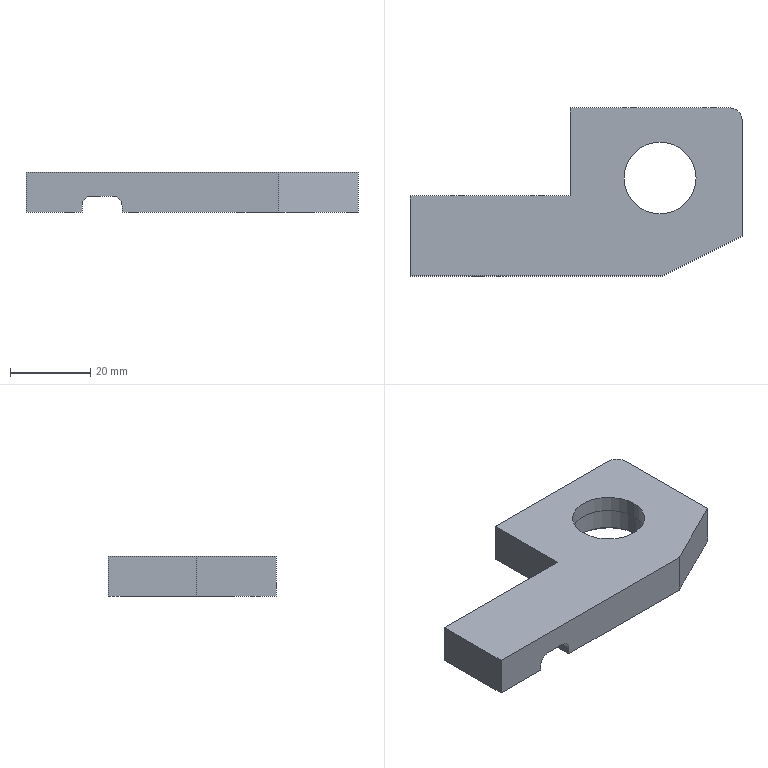Part | NX | features BREP 1 | 1 solid | 47 faces | box 83 x 42 x 10 mm | volume 21101 mm3 | cylinder 19 | cone 14 | plane 14 | commonest cylinder face diameters 3.3 x8 2.5 x4 5 x2 18 x2 19 x2 6 x1
STEP:
#1=CARTESIAN_POINT('',(32.,4.5,-4.5));
#2=VERTEX_POINT('',#1);
#3=CARTESIAN_POINT('',(32.5,4.5,-5.));
#4=VERTEX_POINT('',#3);
#5=CARTESIAN_POINT('',(32.5,4.5,-5.));
#6=DIRECTION('',(0.7071,0.,-0.7071));
#7=VECTOR('',#6,1000.);
#8=LINE('',#5,#7);
#9=EDGE_CURVE('',#2,#4,#8,.T.);
#10=ORIENTED_EDGE('',*,*,#9,.F.);
#11=CARTESIAN_POINT('',(13.,4.5,-4.5));
#12=VERTEX_POINT('',#11);
#13=CARTESIAN_POINT('',(22.5,4.5,-4.5));
#14=DIRECTION('',(0.,0.,-1.));
#15=DIRECTION('',(1.,0.,0.));
#16=AXIS2_PLACEMENT_3D('',#13,#14,#15);
#17=CIRCLE('',#16,9.5);
#18=EDGE_CURVE('',#12,#2,#17,.T.);
#19=ORIENTED_EDGE('',*,*,#18,.F.);
#20=CARTESIAN_POINT('',(12.5,4.5,-5.));
#21=VERTEX_POINT('',#20);
#22=CARTESIAN_POINT('',(12.5,4.5,-5.));
#23=DIRECTION('',(-0.7071,0.,-0.7071));
#24=VECTOR('',#23,1000.);
#25=LINE('',#22,#24);
#26=EDGE_CURVE('',#12,#21,#25,.T.);
#27=ORIENTED_EDGE('',*,*,#26,.T.);
#28=CARTESIAN_POINT('',(22.5,4.5,-5.));
#29=DIRECTION('',(0.,0.,1.));
#30=DIRECTION('',(1.,0.,0.));
#31=AXIS2_PLACEMENT_3D('',#28,#29,#30);
#32=CIRCLE('',#31,10.);
#33=EDGE_CURVE('',#4,#21,#32,.T.);
#34=ORIENTED_EDGE('',*,*,#33,.F.);
#35=EDGE_LOOP('',(#10,#19,#27,#34));
#36=FACE_BOUND('',#35,.T.);
#37=CARTESIAN_POINT('',(22.5,4.5,-5.));
#38=DIRECTION('',(0.,0.,-1.));
#39=DIRECTION('',(-1.,0.,0.));
#40=AXIS2_PLACEMENT_3D('',#37,#38,#39);
#41=CONICAL_SURFACE('',#40,10.,0.7854);
#42=ADVANCED_FACE('',(#36),#41,.F.);
#43=CARTESIAN_POINT('',(-11.75,-15.,2.5));
#44=VERTEX_POINT('',#43);
#45=CARTESIAN_POINT('',(-11.75,-15.,-5.));
#46=VERTEX_POINT('',#45);
#47=CARTESIAN_POINT('',(-11.75,-15.,-5.));
#48=DIRECTION('',(0.,0.,-1.));
#49=VECTOR('',#48,1000.);
#50=LINE('',#47,#49);
#51=EDGE_CURVE('',#44,#46,#50,.T.);
#52=ORIENTED_EDGE('',*,*,#51,.F.);
#53=CARTESIAN_POINT('',(-14.25,-15.,2.5));
#54=VERTEX_POINT('',#53);
#55=CARTESIAN_POINT('',(-13.,-15.,2.5));
#56=DIRECTION('',(0.,0.,-1.));
#57=DIRECTION('',(-1.,0.,0.));
#58=AXIS2_PLACEMENT_3D('',#55,#56,#57);
#59=CIRCLE('',#58,1.25);
#60=EDGE_CURVE('',#54,#44,#59,.T.);
#61=ORIENTED_EDGE('',*,*,#60,.F.);
#62=CARTESIAN_POINT('',(-14.25,-15.,-5.));
#63=VERTEX_POINT('',#62);
#64=CARTESIAN_POINT('',(-14.25,-15.,-5.));
#65=DIRECTION('',(0.,0.,-1.));
#66=VECTOR('',#65,1000.);
#67=LINE('',#64,#66);
#68=EDGE_CURVE('',#54,#63,#67,.T.);
#69=ORIENTED_EDGE('',*,*,#68,.T.);
#70=CARTESIAN_POINT('',(-13.,-15.,-5.));
#71=DIRECTION('',(0.,0.,-1.));
#72=DIRECTION('',(-1.,0.,0.));
#73=AXIS2_PLACEMENT_3D('',#70,#71,#72);
#74=CIRCLE('',#73,1.25);
#75=EDGE_CURVE('',#63,#46,#74,.T.);
#76=ORIENTED_EDGE('',*,*,#75,.T.);
#77=EDGE_LOOP('',(#52,#61,#69,#76));
#78=FACE_BOUND('',#77,.T.);
#79=CARTESIAN_POINT('',(-13.,-15.,-5.));
#80=DIRECTION('',(0.,0.,-1.));
#81=DIRECTION('',(-1.,0.,0.));
#82=AXIS2_PLACEMENT_3D('',#79,#80,#81);
#83=CYLINDRICAL_SURFACE('',#82,1.25);
#84=ADVANCED_FACE('',(#78),#83,.F.);
#85=CARTESIAN_POINT('',(-13.,-15.,3.251));
#86=VERTEX_POINT('',#85);
#87=CARTESIAN_POINT('',(-11.75,-15.,2.5));
#88=DIRECTION('',(0.8572,0.,-0.515));
#89=VECTOR('',#88,1000.);
#90=LINE('',#87,#89);
#91=EDGE_CURVE('',#44,#86,#90,.F.);
#92=ORIENTED_EDGE('',*,*,#91,.T.);
#93=CARTESIAN_POINT('',(-14.25,-15.,2.5));
#94=DIRECTION('',(-0.8572,0.,-0.515));
#95=VECTOR('',#94,1000.);
#96=LINE('',#93,#95);
#97=EDGE_CURVE('',#54,#86,#96,.F.);
#98=ORIENTED_EDGE('',*,*,#97,.F.);
#99=ORIENTED_EDGE('',*,*,#60,.T.);
#100=EDGE_LOOP('',(#92,#98,#99));
#101=FACE_BOUND('',#100,.T.);
#102=CARTESIAN_POINT('',(-13.,-15.,2.5));
#103=DIRECTION('',(0.,0.,-1.));
#104=DIRECTION('',(-1.,0.,0.));
#105=AXIS2_PLACEMENT_3D('',#102,#103,#104);
#106=CONICAL_SURFACE('',#105,1.25,1.03);
#107=ADVANCED_FACE('',(#101),#106,.F.);
#108=CARTESIAN_POINT('',(-27.75,-15.,2.5));
#109=VERTEX_POINT('',#108);
#110=CARTESIAN_POINT('',(-27.75,-15.,-5.));
#111=VERTEX_POINT('',#110);
#112=CARTESIAN_POINT('',(-27.75,-15.,-5.));
#113=DIRECTION('',(0.,0.,-1.));
#114=VECTOR('',#113,1000.);
#115=LINE('',#112,#114);
#116=EDGE_CURVE('',#109,#111,#115,.T.);
#117=ORIENTED_EDGE('',*,*,#116,.F.);
#118=CARTESIAN_POINT('',(-30.25,-15.,2.5));
#119=VERTEX_POINT('',#118);
#120=CARTESIAN_POINT('',(-29.,-15.,2.5));
#121=DIRECTION('',(0.,0.,-1.));
#122=DIRECTION('',(-1.,0.,0.));
#123=AXIS2_PLACEMENT_3D('',#120,#121,#122);
#124=CIRCLE('',#123,1.25);
#125=EDGE_CURVE('',#119,#109,#124,.T.);
#126=ORIENTED_EDGE('',*,*,#125,.F.);
#127=CARTESIAN_POINT('',(-30.25,-15.,-5.));
#128=VERTEX_POINT('',#127);
#129=CARTESIAN_POINT('',(-30.25,-15.,-5.));
#130=DIRECTION('',(0.,0.,-1.));
#131=VECTOR('',#130,1000.);
#132=LINE('',#129,#131);
#133=EDGE_CURVE('',#119,#128,#132,.T.);
#134=ORIENTED_EDGE('',*,*,#133,.T.);
#135=CARTESIAN_POINT('',(-29.,-15.,-5.));
#136=DIRECTION('',(0.,0.,-1.));
#137=DIRECTION('',(-1.,0.,0.));
#138=AXIS2_PLACEMENT_3D('',#135,#136,#137);
#139=CIRCLE('',#138,1.25);
#140=EDGE_CURVE('',#128,#111,#139,.T.);
#141=ORIENTED_EDGE('',*,*,#140,.T.);
#142=EDGE_LOOP('',(#117,#126,#134,#141));
#143=FACE_BOUND('',#142,.T.);
#144=CARTESIAN_POINT('',(-29.,-15.,-5.));
#145=DIRECTION('',(0.,0.,-1.));
#146=DIRECTION('',(-1.,0.,0.));
#147=AXIS2_PLACEMENT_3D('',#144,#145,#146);
#148=CYLINDRICAL_SURFACE('',#147,1.25);
#149=ADVANCED_FACE('',(#143),#148,.F.);
#150=CARTESIAN_POINT('',(-29.,-15.,3.251));
#151=VERTEX_POINT('',#150);
#152=CARTESIAN_POINT('',(-27.75,-15.,2.5));
#153=DIRECTION('',(0.8572,0.,-0.515));
#154=VECTOR('',#153,1000.);
#155=LINE('',#152,#154);
#156=EDGE_CURVE('',#109,#151,#155,.F.);
#157=ORIENTED_EDGE('',*,*,#156,.T.);
#158=CARTESIAN_POINT('',(-30.25,-15.,2.5));
#159=DIRECTION('',(-0.8572,0.,-0.515));
#160=VECTOR('',#159,1000.);
#161=LINE('',#158,#160);
#162=EDGE_CURVE('',#119,#151,#161,.F.);
#163=ORIENTED_EDGE('',*,*,#162,.F.);
#164=ORIENTED_EDGE('',*,*,#125,.T.);
#165=EDGE_LOOP('',(#157,#163,#164));
#166=FACE_BOUND('',#165,.T.);
#167=CARTESIAN_POINT('',(-29.,-15.,2.5));
#168=DIRECTION('',(0.,0.,-1.));
#169=DIRECTION('',(-1.,0.,0.));
#170=AXIS2_PLACEMENT_3D('',#167,#168,#169);
#171=CONICAL_SURFACE('',#170,1.25,1.03);
#172=ADVANCED_FACE('',(#166),#171,.F.);
#173=CARTESIAN_POINT('',(-26.,0.,-3.5));
#174=VERTEX_POINT('',#173);
#175=CARTESIAN_POINT('',(-23.5,0.,-1.));
#176=VERTEX_POINT('',#175);
#177=CARTESIAN_POINT('',(-23.5,0.,-3.5));
#178=DIRECTION('',(0.,1.,0.));
#179=DIRECTION('',(0.,0.,-1.));
#180=AXIS2_PLACEMENT_3D('',#177,#178,#179);
#181=CIRCLE('',#180,2.5);
#182=EDGE_CURVE('',#174,#176,#181,.T.);
#183=ORIENTED_EDGE('',*,*,#182,.T.);
#184=CARTESIAN_POINT('',(-23.5,-20.,-1.));
#185=VERTEX_POINT('',#184);
#186=CARTESIAN_POINT('',(-23.5,-20.,-1.));
#187=DIRECTION('',(0.,1.,0.));
#188=VECTOR('',#187,1000.);
#189=LINE('',#186,#188);
#190=EDGE_CURVE('',#185,#176,#189,.T.);
#191=ORIENTED_EDGE('',*,*,#190,.F.);
#192=CARTESIAN_POINT('',(-26.,-20.,-3.5));
#193=VERTEX_POINT('',#192);
#194=CARTESIAN_POINT('',(-23.5,-20.,-3.5));
#195=DIRECTION('',(0.,1.,0.));
#196=DIRECTION('',(0.,0.,-1.));
#197=AXIS2_PLACEMENT_3D('',#194,#195,#196);
#198=CIRCLE('',#197,2.5);
#199=EDGE_CURVE('',#193,#185,#198,.T.);
#200=ORIENTED_EDGE('',*,*,#199,.F.);
#201=CARTESIAN_POINT('',(-26.,-20.,-3.5));
#202=DIRECTION('',(0.,1.,0.));
#203=VECTOR('',#202,1000.);
#204=LINE('',#201,#203);
#205=EDGE_CURVE('',#193,#174,#204,.T.);
#206=ORIENTED_EDGE('',*,*,#205,.T.);
#207=EDGE_LOOP('',(#183,#191,#200,#206));
#208=FACE_BOUND('',#207,.T.);
#209=CARTESIAN_POINT('',(-23.5,-20.,-3.5));
#210=DIRECTION('',(0.,1.,0.));
#211=DIRECTION('',(0.,0.,1.));
#212=AXIS2_PLACEMENT_3D('',#209,#210,#211);
#213=CYLINDRICAL_SURFACE('',#212,2.5);
#214=ADVANCED_FACE('',(#208),#213,.F.);
#215=CARTESIAN_POINT('',(-18.5,0.,-1.));
#216=VERTEX_POINT('',#215);
#217=CARTESIAN_POINT('',(-18.5,0.,-1.));
#218=DIRECTION('',(1.,0.,0.));
#219=VECTOR('',#218,1000.);
#220=LINE('',#217,#219);
#221=EDGE_CURVE('',#176,#216,#220,.T.);
#222=ORIENTED_EDGE('',*,*,#221,.T.);
#223=CARTESIAN_POINT('',(-18.5,-20.,-1.));
#224=VERTEX_POINT('',#223);
#225=CARTESIAN_POINT('',(-18.5,-20.,-1.));
#226=DIRECTION('',(0.,1.,0.));
#227=VECTOR('',#226,1000.);
#228=LINE('',#225,#227);
#229=EDGE_CURVE('',#224,#216,#228,.T.);
#230=ORIENTED_EDGE('',*,*,#229,.F.);
#231=CARTESIAN_POINT('',(-18.5,-20.,-1.));
#232=DIRECTION('',(1.,0.,0.));
#233=VECTOR('',#232,1000.);
#234=LINE('',#231,#233);
#235=EDGE_CURVE('',#185,#224,#234,.T.);
#236=ORIENTED_EDGE('',*,*,#235,.F.);
#237=ORIENTED_EDGE('',*,*,#190,.T.);
#238=EDGE_LOOP('',(#222,#230,#236,#237));
#239=FACE_BOUND('',#238,.T.);
#240=CARTESIAN_POINT('',(-18.5,-20.,-1.));
#241=DIRECTION('',(0.,0.,1.));
#242=DIRECTION('',(1.,0.,0.));
#243=AXIS2_PLACEMENT_3D('',#240,#241,#242);
#244=PLANE('',#243);
#245=ADVANCED_FACE('',(#239),#244,.F.);
#246=CARTESIAN_POINT('',(-16.,0.,-3.5));
#247=VERTEX_POINT('',#246);
#248=CARTESIAN_POINT('',(-18.5,0.,-3.5));
#249=DIRECTION('',(0.,1.,0.));
#250=DIRECTION('',(0.,0.,-1.));
#251=AXIS2_PLACEMENT_3D('',#248,#249,#250);
#252=CIRCLE('',#251,2.5);
#253=EDGE_CURVE('',#216,#247,#252,.T.);
#254=ORIENTED_EDGE('',*,*,#253,.T.);
#255=CARTESIAN_POINT('',(-16.,-20.,-3.5));
#256=VERTEX_POINT('',#255);
#257=CARTESIAN_POINT('',(-16.,-20.,-3.5));
#258=DIRECTION('',(0.,1.,0.));
#259=VECTOR('',#258,1000.);
#260=LINE('',#257,#259);
#261=EDGE_CURVE('',#256,#247,#260,.T.);
#262=ORIENTED_EDGE('',*,*,#261,.F.);
#263=CARTESIAN_POINT('',(-18.5,-20.,-3.5));
#264=DIRECTION('',(0.,1.,0.));
#265=DIRECTION('',(0.,0.,-1.));
#266=AXIS2_PLACEMENT_3D('',#263,#264,#265);
#267=CIRCLE('',#266,2.5);
#268=EDGE_CURVE('',#224,#256,#267,.T.);
#269=ORIENTED_EDGE('',*,*,#268,.F.);
#270=ORIENTED_EDGE('',*,*,#229,.T.);
#271=EDGE_LOOP('',(#254,#262,#269,#270));
#272=FACE_BOUND('',#271,.T.);
#273=CARTESIAN_POINT('',(-18.5,-20.,-3.5));
#274=DIRECTION('',(0.,1.,0.));
#275=DIRECTION('',(0.,0.,1.));
#276=AXIS2_PLACEMENT_3D('',#273,#274,#275);
#277=CYLINDRICAL_SURFACE('',#276,2.5);
#278=ADVANCED_FACE('',(#272),#277,.F.);
#279=CARTESIAN_POINT('',(-26.,0.,-5.));
#280=VERTEX_POINT('',#279);
#281=CARTESIAN_POINT('',(-26.,0.,-9.));
#282=DIRECTION('',(0.,0.,1.));
#283=VECTOR('',#282,1000.);
#284=LINE('',#281,#283);
#285=EDGE_CURVE('',#280,#174,#284,.T.);
#286=ORIENTED_EDGE('',*,*,#285,.T.);
#287=ORIENTED_EDGE('',*,*,#205,.F.);
#288=CARTESIAN_POINT('',(-26.,-20.,-5.));
#289=VERTEX_POINT('',#288);
#290=CARTESIAN_POINT('',(-26.,-20.,-9.));
#291=DIRECTION('',(0.,0.,1.));
#292=VECTOR('',#291,1000.);
#293=LINE('',#290,#292);
#294=EDGE_CURVE('',#289,#193,#293,.T.);
#295=ORIENTED_EDGE('',*,*,#294,.F.);
#296=CARTESIAN_POINT('',(-26.,0.,-5.));
#297=DIRECTION('',(0.,-1.,0.));
#298=VECTOR('',#297,1000.);
#299=LINE('',#296,#298);
#300=EDGE_CURVE('',#280,#289,#299,.T.);
#301=ORIENTED_EDGE('',*,*,#300,.F.);
#302=EDGE_LOOP('',(#286,#287,#295,#301));
#303=FACE_BOUND('',#302,.T.);
#304=CARTESIAN_POINT('',(-26.,-20.,-9.));
#305=DIRECTION('',(-1.,0.,0.));
#306=DIRECTION('',(0.,0.,1.));
#307=AXIS2_PLACEMENT_3D('',#304,#305,#306);
#308=PLANE('',#307);
#309=ADVANCED_FACE('',(#303),#308,.F.);
#310=CARTESIAN_POINT('',(-16.,-20.,-5.));
#311=VERTEX_POINT('',#310);
#312=CARTESIAN_POINT('',(-16.,-20.,-9.));
#313=DIRECTION('',(0.,0.,-1.));
#314=VECTOR('',#313,1000.);
#315=LINE('',#312,#314);
#316=EDGE_CURVE('',#256,#311,#315,.T.);
#317=ORIENTED_EDGE('',*,*,#316,.F.);
#318=ORIENTED_EDGE('',*,*,#261,.T.);
#319=CARTESIAN_POINT('',(-16.,0.,-5.));
#320=VERTEX_POINT('',#319);
#321=CARTESIAN_POINT('',(-16.,0.,-9.));
#322=DIRECTION('',(0.,0.,-1.));
#323=VECTOR('',#322,1000.);
#324=LINE('',#321,#323);
#325=EDGE_CURVE('',#247,#320,#324,.T.);
#326=ORIENTED_EDGE('',*,*,#325,.T.);
#327=CARTESIAN_POINT('',(-16.,0.,-5.));
#328=DIRECTION('',(0.,1.,0.));
#329=VECTOR('',#328,1000.);
#330=LINE('',#327,#329);
#331=EDGE_CURVE('',#311,#320,#330,.T.);
#332=ORIENTED_EDGE('',*,*,#331,.F.);
#333=EDGE_LOOP('',(#317,#318,#326,#332));
#334=FACE_BOUND('',#333,.T.);
#335=CARTESIAN_POINT('',(-16.,-20.,-9.));
#336=DIRECTION('',(1.,0.,0.));
#337=DIRECTION('',(0.,0.,-1.));
#338=AXIS2_PLACEMENT_3D('',#335,#336,#337);
#339=PLANE('',#338);
#340=ADVANCED_FACE('',(#334),#339,.F.);
#341=CARTESIAN_POINT('',(35.,22.,-1.65));
#342=VERTEX_POINT('',#341);
#343=CARTESIAN_POINT('',(35.,11.9,-1.65));
#344=VERTEX_POINT('',#343);
#345=CARTESIAN_POINT('',(35.,22.,-1.65));
#346=DIRECTION('',(0.,1.,0.));
#347=VECTOR('',#346,1000.);
#348=LINE('',#345,#347);
#349=EDGE_CURVE('',#342,#344,#348,.F.);
#350=ORIENTED_EDGE('',*,*,#349,.T.);
#351=CARTESIAN_POINT('',(35.,11.9,1.65));
#352=VERTEX_POINT('',#351);
#353=CARTESIAN_POINT('',(35.,11.9,0.));
#354=DIRECTION('',(0.,1.,0.));
#355=DIRECTION('',(0.,0.,1.));
#356=AXIS2_PLACEMENT_3D('',#353,#354,#355);
#357=CIRCLE('',#356,1.65);
#358=EDGE_CURVE('',#352,#344,#357,.T.);
#359=ORIENTED_EDGE('',*,*,#358,.F.);
#360=CARTESIAN_POINT('',(35.,22.,1.65));
#361=VERTEX_POINT('',#360);
#362=CARTESIAN_POINT('',(35.,22.,1.65));
#363=DIRECTION('',(0.,1.,0.));
#364=VECTOR('',#363,1000.);
#365=LINE('',#362,#364);
#366=EDGE_CURVE('',#361,#352,#365,.F.);
#367=ORIENTED_EDGE('',*,*,#366,.F.);
#368=CARTESIAN_POINT('',(35.,22.,0.));
#369=DIRECTION('',(0.,1.,0.));
#370=DIRECTION('',(0.,0.,1.));
#371=AXIS2_PLACEMENT_3D('',#368,#369,#370);
#372=CIRCLE('',#371,1.65);
#373=EDGE_CURVE('',#361,#342,#372,.T.);
#374=ORIENTED_EDGE('',*,*,#373,.T.);
#375=EDGE_LOOP('',(#350,#359,#367,#374));
#376=FACE_BOUND('',#375,.T.);
#377=CARTESIAN_POINT('',(35.,22.,0.));
#378=DIRECTION('',(0.,1.,0.));
#379=DIRECTION('',(0.,0.,1.));
#380=AXIS2_PLACEMENT_3D('',#377,#378,#379);
#381=CYLINDRICAL_SURFACE('',#380,1.65);
#382=ADVANCED_FACE('',(#376),#381,.F.);
#383=CARTESIAN_POINT('',(35.,10.909,0.));
#384=VERTEX_POINT('',#383);
#385=CARTESIAN_POINT('',(35.,11.9,-1.65));
#386=DIRECTION('',(0.,0.515,-0.8572));
#387=VECTOR('',#386,1000.);
#388=LINE('',#385,#387);
#389=EDGE_CURVE('',#384,#344,#388,.T.);
#390=ORIENTED_EDGE('',*,*,#389,.F.);
#391=CARTESIAN_POINT('',(35.,11.9,1.65));
#392=DIRECTION('',(0.,0.515,0.8572));
#393=VECTOR('',#392,1000.);
#394=LINE('',#391,#393);
#395=EDGE_CURVE('',#384,#352,#394,.T.);
#396=ORIENTED_EDGE('',*,*,#395,.T.);
#397=ORIENTED_EDGE('',*,*,#358,.T.);
#398=EDGE_LOOP('',(#390,#396,#397));
#399=FACE_BOUND('',#398,.T.);
#400=CARTESIAN_POINT('',(35.,11.9,0.));
#401=DIRECTION('',(0.,1.,0.));
#402=DIRECTION('',(0.,0.,1.));
#403=AXIS2_PLACEMENT_3D('',#400,#401,#402);
#404=CONICAL_SURFACE('',#403,1.65,1.03);
#405=ADVANCED_FACE('',(#399),#404,.F.);
#406=CARTESIAN_POINT('',(15.,22.,-1.65));
#407=VERTEX_POINT('',#406);
#408=CARTESIAN_POINT('',(15.,11.9,-1.65));
#409=VERTEX_POINT('',#408);
#410=CARTESIAN_POINT('',(15.,22.,-1.65));
#411=DIRECTION('',(0.,1.,0.));
#412=VECTOR('',#411,1000.);
#413=LINE('',#410,#412);
#414=EDGE_CURVE('',#407,#409,#413,.F.);
#415=ORIENTED_EDGE('',*,*,#414,.T.);
#416=CARTESIAN_POINT('',(16.543,11.9,-0.5854));
#417=VERTEX_POINT('',#416);
#418=CARTESIAN_POINT('',(15.,11.9,0.));
#419=DIRECTION('',(0.,1.,0.));
#420=DIRECTION('',(0.,0.,1.));
#421=AXIS2_PLACEMENT_3D('',#418,#419,#420);
#422=CIRCLE('',#421,1.65);
#423=EDGE_CURVE('',#417,#409,#422,.T.);
#424=ORIENTED_EDGE('',*,*,#423,.F.);
#425=CARTESIAN_POINT('',(16.543,11.9,0.5854));
#426=VERTEX_POINT('',#425);
#427=CARTESIAN_POINT('',(16.543,11.9,-0.5854));
#428=CARTESIAN_POINT('',(16.684,12.014,-0.2124));
#429=CARTESIAN_POINT('',(16.684,12.014,0.2124));
#430=CARTESIAN_POINT('',(16.543,11.9,0.5854));
#431=B_SPLINE_CURVE_WITH_KNOTS('',3,(#427,#428,#429,#430),.UNSPECIFIED.,.F.,.F.,(4,4),(0.,1.),.UNSPECIFIED.);
#432=EDGE_CURVE('',#417,#426,#431,.T.);
#433=ORIENTED_EDGE('',*,*,#432,.T.);
#434=CARTESIAN_POINT('',(15.,11.9,1.65));
#435=VERTEX_POINT('',#434);
#436=CARTESIAN_POINT('',(15.,11.9,0.));
#437=DIRECTION('',(0.,1.,0.));
#438=DIRECTION('',(0.,0.,1.));
#439=AXIS2_PLACEMENT_3D('',#436,#437,#438);
#440=CIRCLE('',#439,1.65);
#441=EDGE_CURVE('',#435,#426,#440,.T.);
#442=ORIENTED_EDGE('',*,*,#441,.F.);
#443=CARTESIAN_POINT('',(15.,22.,1.65));
#444=VERTEX_POINT('',#443);
#445=CARTESIAN_POINT('',(15.,22.,1.65));
#446=DIRECTION('',(0.,1.,0.));
#447=VECTOR('',#446,1000.);
#448=LINE('',#445,#447);
#449=EDGE_CURVE('',#444,#435,#448,.F.);
#450=ORIENTED_EDGE('',*,*,#449,.F.);
#451=CARTESIAN_POINT('',(15.,22.,0.));
#452=DIRECTION('',(0.,1.,0.));
#453=DIRECTION('',(0.,0.,1.));
#454=AXIS2_PLACEMENT_3D('',#451,#452,#453);
#455=CIRCLE('',#454,1.65);
#456=EDGE_CURVE('',#444,#407,#455,.T.);
#457=ORIENTED_EDGE('',*,*,#456,.T.);
#458=EDGE_LOOP('',(#415,#424,#433,#442,#450,#457));
#459=FACE_BOUND('',#458,.T.);
#460=CARTESIAN_POINT('',(15.,22.,0.));
#461=DIRECTION('',(0.,1.,0.));
#462=DIRECTION('',(0.,0.,1.));
#463=AXIS2_PLACEMENT_3D('',#460,#461,#462);
#464=CYLINDRICAL_SURFACE('',#463,1.65);
#465=ADVANCED_FACE('',(#459),#464,.F.);
#466=CARTESIAN_POINT('',(15.,10.909,0.));
#467=VERTEX_POINT('',#466);
#468=CARTESIAN_POINT('',(15.,11.9,-1.65));
#469=DIRECTION('',(0.,0.515,-0.8572));
#470=VECTOR('',#469,1000.);
#471=LINE('',#468,#470);
#472=EDGE_CURVE('',#467,#409,#471,.T.);
#473=ORIENTED_EDGE('',*,*,#472,.F.);
#474=CARTESIAN_POINT('',(15.,11.9,1.65));
#475=DIRECTION('',(0.,0.515,0.8572));
#476=VECTOR('',#475,1000.);
#477=LINE('',#474,#476);
#478=EDGE_CURVE('',#467,#435,#477,.T.);
#479=ORIENTED_EDGE('',*,*,#478,.T.);
#480=ORIENTED_EDGE('',*,*,#441,.T.);
#481=CARTESIAN_POINT('',(16.543,11.9,-0.5854));
#482=CARTESIAN_POINT('',(16.39,11.777,-0.4109));
#483=CARTESIAN_POINT('',(16.149,11.566,-0.001288));
#484=CARTESIAN_POINT('',(16.389,11.776,0.4098));
#485=CARTESIAN_POINT('',(16.543,11.9,0.5854));
#486=B_SPLINE_CURVE_WITH_KNOTS('',3,(#481,#482,#483,#484,#485),.UNSPECIFIED.,.F.,.F.,(4,1,4),(0.,0.5,1.),.UNSPECIFIED.);
#487=EDGE_CURVE('',#426,#417,#486,.F.);
#488=ORIENTED_EDGE('',*,*,#487,.T.);
#489=ORIENTED_EDGE('',*,*,#423,.T.);
#490=EDGE_LOOP('',(#473,#479,#480,#488,#489));
#491=FACE_BOUND('',#490,.T.);
#492=CARTESIAN_POINT('',(15.,11.9,0.));
#493=DIRECTION('',(0.,1.,0.));
#494=DIRECTION('',(0.,0.,1.));
#495=AXIS2_PLACEMENT_3D('',#492,#493,#494);
#496=CONICAL_SURFACE('',#495,1.65,1.03);
#497=ADVANCED_FACE('',(#491),#496,.F.);
#498=CARTESIAN_POINT('',(43.,19.,5.));
#499=VERTEX_POINT('',#498);
#500=CARTESIAN_POINT('',(40.,22.,5.));
#501=VERTEX_POINT('',#500);
#502=CARTESIAN_POINT('',(40.,19.,5.));
#503=DIRECTION('',(0.,0.,1.));
#504=DIRECTION('',(1.,0.,0.));
#505=AXIS2_PLACEMENT_3D('',#502,#503,#504);
#506=CIRCLE('',#505,3.);
#507=EDGE_CURVE('',#499,#501,#506,.T.);
#508=ORIENTED_EDGE('',*,*,#507,.F.);
#509=CARTESIAN_POINT('',(43.,19.,-5.));
#510=VERTEX_POINT('',#509);
#511=CARTESIAN_POINT('',(43.,19.,5.));
#512=DIRECTION('',(0.,0.,1.));
#513=VECTOR('',#512,1000.);
#514=LINE('',#511,#513);
#515=EDGE_CURVE('',#510,#499,#514,.T.);
#516=ORIENTED_EDGE('',*,*,#515,.F.);
#517=CARTESIAN_POINT('',(40.,22.,-5.));
#518=VERTEX_POINT('',#517);
#519=CARTESIAN_POINT('',(40.,19.,-5.));
#520=DIRECTION('',(0.,0.,-1.));
#521=DIRECTION('',(1.,0.,0.));
#522=AXIS2_PLACEMENT_3D('',#519,#520,#521);
#523=CIRCLE('',#522,3.);
#524=EDGE_CURVE('',#518,#510,#523,.T.);
#525=ORIENTED_EDGE('',*,*,#524,.F.);
#526=CARTESIAN_POINT('',(40.,22.,5.));
#527=DIRECTION('',(0.,0.,-1.));
#528=VECTOR('',#527,1000.);
#529=LINE('',#526,#528);
#530=EDGE_CURVE('',#501,#518,#529,.T.);
#531=ORIENTED_EDGE('',*,*,#530,.F.);
#532=EDGE_LOOP('',(#508,#516,#525,#531));
#533=FACE_BOUND('',#532,.T.);
#534=CARTESIAN_POINT('',(40.,19.,5.));
#535=DIRECTION('',(0.,0.,-1.));
#536=DIRECTION('',(-1.,0.,0.));
#537=AXIS2_PLACEMENT_3D('',#534,#535,#536);
#538=CYLINDRICAL_SURFACE('',#537,3.);
#539=ADVANCED_FACE('',(#533),#538,.T.);
#540=CARTESIAN_POINT('',(13.5,4.5,5.));
#541=VERTEX_POINT('',#540);
#542=CARTESIAN_POINT('',(13.5,4.5,1.));
#543=VERTEX_POINT('',#542);
#544=CARTESIAN_POINT('',(13.5,4.5,-5.));
#545=DIRECTION('',(0.,0.,1.));
#546=VECTOR('',#545,1000.);
#547=LINE('',#544,#546);
#548=EDGE_CURVE('',#541,#543,#547,.F.);
#549=ORIENTED_EDGE('',*,*,#548,.T.);
#550=CARTESIAN_POINT('',(31.5,4.5,1.));
#551=VERTEX_POINT('',#550);
#552=CARTESIAN_POINT('',(22.5,4.5,1.));
#553=DIRECTION('',(0.,0.,1.));
#554=DIRECTION('',(1.,0.,0.));
#555=AXIS2_PLACEMENT_3D('',#552,#553,#554);
#556=CIRCLE('',#555,9.);
#557=EDGE_CURVE('',#551,#543,#556,.T.);
#558=ORIENTED_EDGE('',*,*,#557,.F.);
#559=CARTESIAN_POINT('',(31.5,4.5,5.));
#560=VERTEX_POINT('',#559);
#561=CARTESIAN_POINT('',(31.5,4.5,-5.));
#562=DIRECTION('',(0.,0.,1.));
#563=VECTOR('',#562,1000.);
#564=LINE('',#561,#563);
#565=EDGE_CURVE('',#560,#551,#564,.F.);
#566=ORIENTED_EDGE('',*,*,#565,.F.);
#567=CARTESIAN_POINT('',(22.5,4.5,5.));
#568=DIRECTION('',(0.,0.,1.));
#569=DIRECTION('',(1.,0.,0.));
#570=AXIS2_PLACEMENT_3D('',#567,#568,#569);
#571=CIRCLE('',#570,9.);
#572=EDGE_CURVE('',#560,#541,#571,.T.);
#573=ORIENTED_EDGE('',*,*,#572,.T.);
#574=EDGE_LOOP('',(#549,#558,#566,#573));
#575=FACE_BOUND('',#574,.T.);
#576=CARTESIAN_POINT('',(22.5,4.5,-5.));
#577=DIRECTION('',(0.,0.,1.));
#578=DIRECTION('',(1.,0.,0.));
#579=AXIS2_PLACEMENT_3D('',#576,#577,#578);
#580=CYLINDRICAL_SURFACE('',#579,9.);
#581=ADVANCED_FACE('',(#575),#580,.F.);
#582=CARTESIAN_POINT('',(13.,4.5,1.));
#583=VERTEX_POINT('',#582);
#584=CARTESIAN_POINT('',(32.,4.5,1.));
#585=VERTEX_POINT('',#584);
#586=CARTESIAN_POINT('',(22.5,4.5,1.));
#587=DIRECTION('',(0.,0.,1.));
#588=DIRECTION('',(1.,0.,0.));
#589=AXIS2_PLACEMENT_3D('',#586,#587,#588);
#590=CIRCLE('',#589,9.5);
#591=EDGE_CURVE('',#583,#585,#590,.T.);
#592=ORIENTED_EDGE('',*,*,#591,.F.);
#593=CARTESIAN_POINT('',(22.5,4.5,1.));
#594=DIRECTION('',(0.,0.,1.));
#595=DIRECTION('',(1.,0.,0.));
#596=AXIS2_PLACEMENT_3D('',#593,#594,#595);
#597=CIRCLE('',#596,9.5);
#598=EDGE_CURVE('',#585,#583,#597,.T.);
#599=ORIENTED_EDGE('',*,*,#598,.F.);
#600=EDGE_LOOP('',(#592,#599));
#601=FACE_BOUND('',#600,.T.);
#602=ORIENTED_EDGE('',*,*,#557,.T.);
#603=CARTESIAN_POINT('',(22.5,4.5,1.));
#604=DIRECTION('',(0.,0.,1.));
#605=DIRECTION('',(1.,0.,0.));
#606=AXIS2_PLACEMENT_3D('',#603,#604,#605);
#607=CIRCLE('',#606,9.);
#608=EDGE_CURVE('',#543,#551,#607,.T.);
#609=ORIENTED_EDGE('',*,*,#608,.T.);
#610=EDGE_LOOP('',(#602,#609));
#611=FACE_BOUND('',#610,.T.);
#612=CARTESIAN_POINT('',(22.5,4.5,1.));
#613=DIRECTION('',(0.,0.,1.));
#614=DIRECTION('',(1.,0.,0.));
#615=AXIS2_PLACEMENT_3D('',#612,#613,#614);
#616=PLANE('',#615);
#617=ADVANCED_FACE('',(#601,#611),#616,.F.);
#618=ORIENTED_EDGE('',*,*,#432,.F.);
#619=ORIENTED_EDGE('',*,*,#487,.F.);
#620=EDGE_LOOP('',(#618,#619));
#621=FACE_BOUND('',#620,.T.);
#622=CARTESIAN_POINT('',(32.,4.5,1.));
#623=DIRECTION('',(0.,0.,-1.));
#624=VECTOR('',#623,1000.);
#625=LINE('',#622,#624);
#626=EDGE_CURVE('',#585,#2,#625,.T.);
#627=ORIENTED_EDGE('',*,*,#626,.F.);
#628=ORIENTED_EDGE('',*,*,#598,.T.);
#629=CARTESIAN_POINT('',(13.,4.5,1.));
#630=DIRECTION('',(0.,0.,-1.));
#631=VECTOR('',#630,1000.);
#632=LINE('',#629,#631);
#633=EDGE_CURVE('',#583,#12,#632,.T.);
#634=ORIENTED_EDGE('',*,*,#633,.T.);
#635=ORIENTED_EDGE('',*,*,#18,.T.);
#636=EDGE_LOOP('',(#627,#628,#634,#635));
#637=FACE_BOUND('',#636,.T.);
#638=CARTESIAN_POINT('',(22.5,4.5,1.));
#639=DIRECTION('',(0.,0.,-1.));
#640=DIRECTION('',(-1.,0.,0.));
#641=AXIS2_PLACEMENT_3D('',#638,#639,#640);
#642=CYLINDRICAL_SURFACE('',#641,9.5);
#643=ADVANCED_FACE('',(#621,#637),#642,.F.);
#644=CARTESIAN_POINT('',(23.,-20.,5.));
#645=VERTEX_POINT('',#644);
#646=CARTESIAN_POINT('',(43.,-10.,5.));
#647=VERTEX_POINT('',#646);
#648=CARTESIAN_POINT('',(12.6,-25.2,5.));
#649=DIRECTION('',(0.8944,0.4472,0.));
#650=VECTOR('',#649,1000.);
#651=LINE('',#648,#650);
#652=EDGE_CURVE('',#645,#647,#651,.T.);
#653=ORIENTED_EDGE('',*,*,#652,.F.);
#654=CARTESIAN_POINT('',(23.,-20.,-5.));
#655=VERTEX_POINT('',#654);
#656=CARTESIAN_POINT('',(23.,-20.,5.));
#657=DIRECTION('',(0.,0.,1.));
#658=VECTOR('',#657,1000.);
#659=LINE('',#656,#658);
#660=EDGE_CURVE('',#655,#645,#659,.T.);
#661=ORIENTED_EDGE('',*,*,#660,.F.);
#662=CARTESIAN_POINT('',(43.,-10.,-5.));
#663=VERTEX_POINT('',#662);
#664=CARTESIAN_POINT('',(43.,-10.,-5.));
#665=DIRECTION('',(-0.8944,-0.4472,0.));
#666=VECTOR('',#665,1000.);
#667=LINE('',#664,#666);
#668=EDGE_CURVE('',#663,#655,#667,.T.);
#669=ORIENTED_EDGE('',*,*,#668,.F.);
#670=CARTESIAN_POINT('',(43.,-10.,5.));
#671=DIRECTION('',(0.,0.,-1.));
#672=VECTOR('',#671,1000.);
#673=LINE('',#670,#672);
#674=EDGE_CURVE('',#647,#663,#673,.T.);
#675=ORIENTED_EDGE('',*,*,#674,.F.);
#676=EDGE_LOOP('',(#653,#661,#669,#675));
#677=FACE_BOUND('',#676,.T.);
#678=CARTESIAN_POINT('',(43.,-10.,5.));
#679=DIRECTION('',(-0.4472,0.8944,0.));
#680=DIRECTION('',(0.,0.,-1.));
#681=AXIS2_PLACEMENT_3D('',#678,#679,#680);
#682=PLANE('',#681);
#683=ADVANCED_FACE('',(#677),#682,.F.);
#684=CARTESIAN_POINT('',(-8.,0.,-1.65));
#685=VERTEX_POINT('',#684);
#686=CARTESIAN_POINT('',(-8.,-12.1,-1.65));
#687=VERTEX_POINT('',#686);
#688=CARTESIAN_POINT('',(-8.,0.,-1.65));
#689=DIRECTION('',(0.,1.,0.));
#690=VECTOR('',#689,1000.);
#691=LINE('',#688,#690);
#692=EDGE_CURVE('',#685,#687,#691,.F.);
#693=ORIENTED_EDGE('',*,*,#692,.T.);
#694=CARTESIAN_POINT('',(-8.,-12.1,1.65));
#695=VERTEX_POINT('',#694);
#696=CARTESIAN_POINT('',(-8.,-12.1,0.));
#697=DIRECTION('',(0.,1.,0.));
#698=DIRECTION('',(0.,0.,1.));
#699=AXIS2_PLACEMENT_3D('',#696,#697,#698);
#700=CIRCLE('',#699,1.65);
#701=EDGE_CURVE('',#695,#687,#700,.T.);
#702=ORIENTED_EDGE('',*,*,#701,.F.);
#703=CARTESIAN_POINT('',(-8.,0.,1.65));
#704=VERTEX_POINT('',#703);
#705=CARTESIAN_POINT('',(-8.,0.,1.65));
#706=DIRECTION('',(0.,1.,0.));
#707=VECTOR('',#706,1000.);
#708=LINE('',#705,#707);
#709=EDGE_CURVE('',#704,#695,#708,.F.);
#710=ORIENTED_EDGE('',*,*,#709,.F.);
#711=CARTESIAN_POINT('',(-8.,0.,0.));
#712=DIRECTION('',(0.,1.,0.));
#713=DIRECTION('',(0.,0.,1.));
#714=AXIS2_PLACEMENT_3D('',#711,#712,#713);
#715=CIRCLE('',#714,1.65);
#716=EDGE_CURVE('',#704,#685,#715,.T.);
#717=ORIENTED_EDGE('',*,*,#716,.T.);
#718=EDGE_LOOP('',(#693,#702,#710,#717));
#719=FACE_BOUND('',#718,.T.);
#720=CARTESIAN_POINT('',(-8.,0.,0.));
#721=DIRECTION('',(0.,1.,0.));
#722=DIRECTION('',(0.,0.,1.));
#723=AXIS2_PLACEMENT_3D('',#720,#721,#722);
#724=CYLINDRICAL_SURFACE('',#723,1.65);
#725=ADVANCED_FACE('',(#719),#724,.F.);
#726=CARTESIAN_POINT('',(-8.,-13.091,0.));
#727=VERTEX_POINT('',#726);
#728=CARTESIAN_POINT('',(-8.,-12.1,-1.65));
#729=DIRECTION('',(0.,0.515,-0.8572));
#730=VECTOR('',#729,1000.);
#731=LINE('',#728,#730);
#732=EDGE_CURVE('',#727,#687,#731,.T.);
#733=ORIENTED_EDGE('',*,*,#732,.F.);
#734=CARTESIAN_POINT('',(-8.,-12.1,1.65));
#735=DIRECTION('',(0.,0.515,0.8572));
#736=VECTOR('',#735,1000.);
#737=LINE('',#734,#736);
#738=EDGE_CURVE('',#727,#695,#737,.T.);
#739=ORIENTED_EDGE('',*,*,#738,.T.);
#740=ORIENTED_EDGE('',*,*,#701,.T.);
#741=EDGE_LOOP('',(#733,#739,#740));
#742=FACE_BOUND('',#741,.T.);
#743=CARTESIAN_POINT('',(-8.,-12.1,0.));
#744=DIRECTION('',(0.,1.,0.));
#745=DIRECTION('',(0.,0.,1.));
#746=AXIS2_PLACEMENT_3D('',#743,#744,#745);
#747=CONICAL_SURFACE('',#746,1.65,1.03);
#748=ADVANCED_FACE('',(#742),#747,.F.);
#749=CARTESIAN_POINT('',(-28.,0.,-1.65));
#750=VERTEX_POINT('',#749);
#751=CARTESIAN_POINT('',(-28.,-12.1,-1.65));
#752=VERTEX_POINT('',#751);
#753=CARTESIAN_POINT('',(-28.,0.,-1.65));
#754=DIRECTION('',(0.,1.,0.));
#755=VECTOR('',#754,1000.);
#756=LINE('',#753,#755);
#757=EDGE_CURVE('',#750,#752,#756,.F.);
#758=ORIENTED_EDGE('',*,*,#757,.T.);
#759=CARTESIAN_POINT('',(-28.,-12.1,1.65));
#760=VERTEX_POINT('',#759);
#761=CARTESIAN_POINT('',(-28.,-12.1,0.));
#762=DIRECTION('',(0.,1.,0.));
#763=DIRECTION('',(0.,0.,1.));
#764=AXIS2_PLACEMENT_3D('',#761,#762,#763);
#765=CIRCLE('',#764,1.65);
#766=EDGE_CURVE('',#760,#752,#765,.T.);
#767=ORIENTED_EDGE('',*,*,#766,.F.);
#768=CARTESIAN_POINT('',(-28.,0.,1.65));
#769=VERTEX_POINT('',#768);
#770=CARTESIAN_POINT('',(-28.,0.,1.65));
#771=DIRECTION('',(0.,1.,0.));
#772=VECTOR('',#771,1000.);
#773=LINE('',#770,#772);
#774=EDGE_CURVE('',#769,#760,#773,.F.);
#775=ORIENTED_EDGE('',*,*,#774,.F.);
#776=CARTESIAN_POINT('',(-28.,0.,0.));
#777=DIRECTION('',(0.,1.,0.));
#778=DIRECTION('',(0.,0.,1.));
#779=AXIS2_PLACEMENT_3D('',#776,#777,#778);
#780=CIRCLE('',#779,1.65);
#781=EDGE_CURVE('',#769,#750,#780,.T.);
#782=ORIENTED_EDGE('',*,*,#781,.T.);
#783=EDGE_LOOP('',(#758,#767,#775,#782));
#784=FACE_BOUND('',#783,.T.);
#785=CARTESIAN_POINT('',(-28.,0.,0.));
#786=DIRECTION('',(0.,1.,0.));
#787=DIRECTION('',(0.,0.,1.));
#788=AXIS2_PLACEMENT_3D('',#785,#786,#787);
#789=CYLINDRICAL_SURFACE('',#788,1.65);
#790=ADVANCED_FACE('',(#784),#789,.F.);
#791=CARTESIAN_POINT('',(-28.,-13.091,0.));
#792=VERTEX_POINT('',#791);
#793=CARTESIAN_POINT('',(-28.,-12.1,-1.65));
#794=DIRECTION('',(0.,0.515,-0.8572));
#795=VECTOR('',#794,1000.);
#796=LINE('',#793,#795);
#797=EDGE_CURVE('',#792,#752,#796,.T.);
#798=ORIENTED_EDGE('',*,*,#797,.F.);
#799=CARTESIAN_POINT('',(-28.,-12.1,1.65));
#800=DIRECTION('',(0.,0.515,0.8572));
#801=VECTOR('',#800,1000.);
#802=LINE('',#799,#801);
#803=EDGE_CURVE('',#792,#760,#802,.T.);
#804=ORIENTED_EDGE('',*,*,#803,.T.);
#805=ORIENTED_EDGE('',*,*,#766,.T.);
#806=EDGE_LOOP('',(#798,#804,#805));
#807=FACE_BOUND('',#806,.T.);
#808=CARTESIAN_POINT('',(-28.,-12.1,0.));
#809=DIRECTION('',(0.,1.,0.));
#810=DIRECTION('',(0.,0.,1.));
#811=AXIS2_PLACEMENT_3D('',#808,#809,#810);
#812=CONICAL_SURFACE('',#811,1.65,1.03);
#813=ADVANCED_FACE('',(#807),#812,.F.);
#814=CARTESIAN_POINT('',(-40.,0.,-5.));
#815=VERTEX_POINT('',#814);
#816=CARTESIAN_POINT('',(-40.,0.,-5.));
#817=DIRECTION('',(-1.,0.,0.));
#818=VECTOR('',#817,1000.);
#819=LINE('',#816,#818);
#820=EDGE_CURVE('',#280,#815,#819,.T.);
#821=ORIENTED_EDGE('',*,*,#820,.F.);
#822=ORIENTED_EDGE('',*,*,#300,.T.);
#823=CARTESIAN_POINT('',(-40.,-20.,-5.));
#824=VERTEX_POINT('',#823);
#825=CARTESIAN_POINT('',(43.,-20.,-5.));
#826=DIRECTION('',(1.,0.,0.));
#827=VECTOR('',#826,1000.);
#828=LINE('',#825,#827);
#829=EDGE_CURVE('',#824,#289,#828,.T.);
#830=ORIENTED_EDGE('',*,*,#829,.F.);
#831=CARTESIAN_POINT('',(-40.,-20.,-5.));
#832=DIRECTION('',(0.,-1.,0.));
#833=VECTOR('',#832,1000.);
#834=LINE('',#831,#833);
#835=EDGE_CURVE('',#815,#824,#834,.T.);
#836=ORIENTED_EDGE('',*,*,#835,.F.);
#837=EDGE_LOOP('',(#821,#822,#830,#836));
#838=FACE_BOUND('',#837,.T.);
#839=ORIENTED_EDGE('',*,*,#140,.F.);
#840=CARTESIAN_POINT('',(-29.,-15.,-5.));
#841=DIRECTION('',(0.,0.,-1.));
#842=DIRECTION('',(-1.,0.,0.));
#843=AXIS2_PLACEMENT_3D('',#840,#841,#842);
#844=CIRCLE('',#843,1.25);
#845=EDGE_CURVE('',#111,#128,#844,.T.);
#846=ORIENTED_EDGE('',*,*,#845,.F.);
#847=EDGE_LOOP('',(#839,#846));
#848=FACE_BOUND('',#847,.T.);
#849=CARTESIAN_POINT('',(0.,0.,-5.));
#850=DIRECTION('',(0.,0.,1.));
#851=DIRECTION('',(1.,0.,0.));
#852=AXIS2_PLACEMENT_3D('',#849,#850,#851);
#853=PLANE('',#852);
#854=ADVANCED_FACE('',(#838,#848),#853,.F.);
#855=CARTESIAN_POINT('',(43.,22.,5.));
#856=DIRECTION('',(0.,1.,0.));
#857=VECTOR('',#856,1000.);
#858=LINE('',#855,#857);
#859=EDGE_CURVE('',#647,#499,#858,.T.);
#860=ORIENTED_EDGE('',*,*,#859,.T.);
#861=ORIENTED_EDGE('',*,*,#507,.T.);
#862=CARTESIAN_POINT('',(0.,22.,5.));
#863=VERTEX_POINT('',#862);
#864=CARTESIAN_POINT('',(0.,22.,5.));
#865=DIRECTION('',(-1.,0.,0.));
#866=VECTOR('',#865,1000.);
#867=LINE('',#864,#866);
#868=EDGE_CURVE('',#501,#863,#867,.T.);
#869=ORIENTED_EDGE('',*,*,#868,.T.);
#870=CARTESIAN_POINT('',(0.,0.,5.));
#871=VERTEX_POINT('',#870);
#872=CARTESIAN_POINT('',(0.,0.,5.));
#873=DIRECTION('',(0.,-1.,0.));
#874=VECTOR('',#873,1000.);
#875=LINE('',#872,#874);
#876=EDGE_CURVE('',#863,#871,#875,.T.);
#877=ORIENTED_EDGE('',*,*,#876,.T.);
#878=CARTESIAN_POINT('',(-40.,0.,5.));
#879=VERTEX_POINT('',#878);
#880=CARTESIAN_POINT('',(-40.,0.,5.));
#881=DIRECTION('',(-1.,0.,0.));
#882=VECTOR('',#881,1000.);
#883=LINE('',#880,#882);
#884=EDGE_CURVE('',#871,#879,#883,.T.);
#885=ORIENTED_EDGE('',*,*,#884,.T.);
#886=CARTESIAN_POINT('',(-40.,-20.,5.));
#887=VERTEX_POINT('',#886);
#888=CARTESIAN_POINT('',(-40.,-20.,5.));
#889=DIRECTION('',(0.,-1.,0.));
#890=VECTOR('',#889,1000.);
#891=LINE('',#888,#890);
#892=EDGE_CURVE('',#879,#887,#891,.T.);
#893=ORIENTED_EDGE('',*,*,#892,.T.);
#894=CARTESIAN_POINT('',(43.,-20.,5.));
#895=DIRECTION('',(1.,0.,0.));
#896=VECTOR('',#895,1000.);
#897=LINE('',#894,#896);
#898=EDGE_CURVE('',#887,#645,#897,.T.);
#899=ORIENTED_EDGE('',*,*,#898,.T.);
#900=ORIENTED_EDGE('',*,*,#652,.T.);
#901=EDGE_LOOP('',(#860,#861,#869,#877,#885,#893,#899,#900));
#902=FACE_BOUND('',#901,.T.);
#903=ORIENTED_EDGE('',*,*,#572,.F.);
#904=CARTESIAN_POINT('',(22.5,4.5,5.));
#905=DIRECTION('',(0.,0.,1.));
#906=DIRECTION('',(1.,0.,0.));
#907=AXIS2_PLACEMENT_3D('',#904,#905,#906);
#908=CIRCLE('',#907,9.);
#909=EDGE_CURVE('',#541,#560,#908,.T.);
#910=ORIENTED_EDGE('',*,*,#909,.F.);
#911=EDGE_LOOP('',(#903,#910));
#912=FACE_BOUND('',#911,.T.);
#913=CARTESIAN_POINT('',(0.,0.,5.));
#914=DIRECTION('',(0.,0.,1.));
#915=DIRECTION('',(1.,0.,0.));
#916=AXIS2_PLACEMENT_3D('',#913,#914,#915);
#917=PLANE('',#916);
#918=ADVANCED_FACE('',(#902,#912),#917,.T.);
#919=CARTESIAN_POINT('',(0.,22.,-5.));
#920=VERTEX_POINT('',#919);
#921=CARTESIAN_POINT('',(0.,0.,-5.));
#922=VERTEX_POINT('',#921);
#923=CARTESIAN_POINT('',(0.,0.,-5.));
#924=DIRECTION('',(0.,-1.,0.));
#925=VECTOR('',#924,1000.);
#926=LINE('',#923,#925);
#927=EDGE_CURVE('',#920,#922,#926,.T.);
#928=ORIENTED_EDGE('',*,*,#927,.T.);
#929=CARTESIAN_POINT('',(0.,0.,5.));
#930=DIRECTION('',(0.,0.,-1.));
#931=VECTOR('',#930,1000.);
#932=LINE('',#929,#931);
#933=EDGE_CURVE('',#871,#922,#932,.T.);
#934=ORIENTED_EDGE('',*,*,#933,.F.);
#935=ORIENTED_EDGE('',*,*,#876,.F.);
#936=CARTESIAN_POINT('',(0.,22.,5.));
#937=DIRECTION('',(0.,0.,-1.));
#938=VECTOR('',#937,1000.);
#939=LINE('',#936,#938);
#940=EDGE_CURVE('',#863,#920,#939,.T.);
#941=ORIENTED_EDGE('',*,*,#940,.T.);
#942=EDGE_LOOP('',(#928,#934,#935,#941));
#943=FACE_BOUND('',#942,.T.);
#944=CARTESIAN_POINT('',(0.,0.,5.));
#945=DIRECTION('',(1.,0.,0.));
#946=DIRECTION('',(0.,0.,-1.));
#947=AXIS2_PLACEMENT_3D('',#944,#945,#946);
#948=PLANE('',#947);
#949=ADVANCED_FACE('',(#943),#948,.F.);
#950=ORIENTED_EDGE('',*,*,#868,.F.);
#951=ORIENTED_EDGE('',*,*,#530,.T.);
#952=CARTESIAN_POINT('',(0.,22.,-5.));
#953=DIRECTION('',(-1.,0.,0.));
#954=VECTOR('',#953,1000.);
#955=LINE('',#952,#954);
#956=EDGE_CURVE('',#518,#920,#955,.T.);
#957=ORIENTED_EDGE('',*,*,#956,.T.);
#958=ORIENTED_EDGE('',*,*,#940,.F.);
#959=EDGE_LOOP('',(#950,#951,#957,#958));
#960=FACE_BOUND('',#959,.T.);
#961=ORIENTED_EDGE('',*,*,#456,.F.);
#962=CARTESIAN_POINT('',(15.,22.,0.));
#963=DIRECTION('',(0.,1.,0.));
#964=DIRECTION('',(0.,0.,1.));
#965=AXIS2_PLACEMENT_3D('',#962,#963,#964);
#966=CIRCLE('',#965,1.65);
#967=EDGE_CURVE('',#407,#444,#966,.T.);
#968=ORIENTED_EDGE('',*,*,#967,.F.);
#969=EDGE_LOOP('',(#961,#968));
#970=FACE_BOUND('',#969,.T.);
#971=ORIENTED_EDGE('',*,*,#373,.F.);
#972=CARTESIAN_POINT('',(35.,22.,0.));
#973=DIRECTION('',(0.,1.,0.));
#974=DIRECTION('',(0.,0.,1.));
#975=AXIS2_PLACEMENT_3D('',#972,#973,#974);
#976=CIRCLE('',#975,1.65);
#977=EDGE_CURVE('',#342,#361,#976,.T.);
#978=ORIENTED_EDGE('',*,*,#977,.F.);
#979=EDGE_LOOP('',(#971,#978));
#980=FACE_BOUND('',#979,.T.);
#981=CARTESIAN_POINT('',(0.,22.,5.));
#982=DIRECTION('',(0.,-1.,0.));
#983=DIRECTION('',(0.,0.,-1.));
#984=AXIS2_PLACEMENT_3D('',#981,#982,#983);
#985=PLANE('',#984);
#986=ADVANCED_FACE('',(#960,#970,#980),#985,.F.);
#987=CARTESIAN_POINT('',(43.,22.,-5.));
#988=DIRECTION('',(0.,1.,0.));
#989=VECTOR('',#988,1000.);
#990=LINE('',#987,#989);
#991=EDGE_CURVE('',#663,#510,#990,.T.);
#992=ORIENTED_EDGE('',*,*,#991,.T.);
#993=ORIENTED_EDGE('',*,*,#515,.T.);
#994=ORIENTED_EDGE('',*,*,#859,.F.);
#995=ORIENTED_EDGE('',*,*,#674,.T.);
#996=EDGE_LOOP('',(#992,#993,#994,#995));
#997=FACE_BOUND('',#996,.T.);
#998=CARTESIAN_POINT('',(43.,22.,5.));
#999=DIRECTION('',(-1.,0.,0.));
#1000=DIRECTION('',(0.,0.,1.));
#1001=AXIS2_PLACEMENT_3D('',#998,#999,#1000);
#1002=PLANE('',#1001);
#1003=ADVANCED_FACE('',(#997),#1002,.F.);
#1004=ORIENTED_EDGE('',*,*,#268,.T.);
#1005=ORIENTED_EDGE('',*,*,#316,.T.);
#1006=CARTESIAN_POINT('',(43.,-20.,-5.));
#1007=DIRECTION('',(1.,0.,0.));
#1008=VECTOR('',#1007,1000.);
#1009=LINE('',#1006,#1008);
#1010=EDGE_CURVE('',#311,#655,#1009,.T.);
#1011=ORIENTED_EDGE('',*,*,#1010,.T.);
#1012=ORIENTED_EDGE('',*,*,#660,.T.);
#1013=ORIENTED_EDGE('',*,*,#898,.F.);
#1014=CARTESIAN_POINT('',(-40.,-20.,5.));
#1015=DIRECTION('',(0.,0.,-1.));
#1016=VECTOR('',#1015,1000.);
#1017=LINE('',#1014,#1016);
#1018=EDGE_CURVE('',#887,#824,#1017,.T.);
#1019=ORIENTED_EDGE('',*,*,#1018,.T.);
#1020=ORIENTED_EDGE('',*,*,#829,.T.);
#1021=ORIENTED_EDGE('',*,*,#294,.T.);
#1022=ORIENTED_EDGE('',*,*,#199,.T.);
#1023=ORIENTED_EDGE('',*,*,#235,.T.);
#1024=EDGE_LOOP('',(#1004,#1005,#1011,#1012,#1013,#1019,#1020,#1021,#1022,#1023));
#1025=FACE_BOUND('',#1024,.T.);
#1026=CARTESIAN_POINT('',(43.,-20.,5.));
#1027=DIRECTION('',(0.,1.,0.));
#1028=DIRECTION('',(-1.,0.,0.));
#1029=AXIS2_PLACEMENT_3D('',#1026,#1027,#1028);
#1030=PLANE('',#1029);
#1031=ADVANCED_FACE('',(#1025),#1030,.F.);
#1032=ORIENTED_EDGE('',*,*,#835,.T.);
#1033=ORIENTED_EDGE('',*,*,#1018,.F.);
#1034=ORIENTED_EDGE('',*,*,#892,.F.);
#1035=CARTESIAN_POINT('',(-40.,0.,5.));
#1036=DIRECTION('',(0.,0.,-1.));
#1037=VECTOR('',#1036,1000.);
#1038=LINE('',#1035,#1037);
#1039=EDGE_CURVE('',#879,#815,#1038,.T.);
#1040=ORIENTED_EDGE('',*,*,#1039,.T.);
#1041=EDGE_LOOP('',(#1032,#1033,#1034,#1040));
#1042=FACE_BOUND('',#1041,.T.);
#1043=CARTESIAN_POINT('',(-40.,-20.,5.));
#1044=DIRECTION('',(1.,0.,0.));
#1045=DIRECTION('',(0.,1.,0.));
#1046=AXIS2_PLACEMENT_3D('',#1043,#1044,#1045);
#1047=PLANE('',#1046);
#1048=ADVANCED_FACE('',(#1042),#1047,.F.);
#1049=CARTESIAN_POINT('',(-40.,0.,-5.));
#1050=DIRECTION('',(-1.,0.,0.));
#1051=VECTOR('',#1050,1000.);
#1052=LINE('',#1049,#1051);
#1053=EDGE_CURVE('',#922,#320,#1052,.T.);
#1054=ORIENTED_EDGE('',*,*,#1053,.T.);
#1055=ORIENTED_EDGE('',*,*,#325,.F.);
#1056=ORIENTED_EDGE('',*,*,#253,.F.);
#1057=ORIENTED_EDGE('',*,*,#221,.F.);
#1058=ORIENTED_EDGE('',*,*,#182,.F.);
#1059=ORIENTED_EDGE('',*,*,#285,.F.);
#1060=ORIENTED_EDGE('',*,*,#820,.T.);
#1061=ORIENTED_EDGE('',*,*,#1039,.F.);
#1062=ORIENTED_EDGE('',*,*,#884,.F.);
#1063=ORIENTED_EDGE('',*,*,#933,.T.);
#1064=EDGE_LOOP('',(#1054,#1055,#1056,#1057,#1058,#1059,#1060,#1061,#1062,#1063));
#1065=FACE_BOUND('',#1064,.T.);
#1066=ORIENTED_EDGE('',*,*,#781,.F.);
#1067=CARTESIAN_POINT('',(-28.,0.,0.));
#1068=DIRECTION('',(0.,1.,0.));
#1069=DIRECTION('',(0.,0.,1.));
#1070=AXIS2_PLACEMENT_3D('',#1067,#1068,#1069);
#1071=CIRCLE('',#1070,1.65);
#1072=EDGE_CURVE('',#750,#769,#1071,.T.);
#1073=ORIENTED_EDGE('',*,*,#1072,.F.);
#1074=EDGE_LOOP('',(#1066,#1073));
#1075=FACE_BOUND('',#1074,.T.);
#1076=ORIENTED_EDGE('',*,*,#716,.F.);
#1077=CARTESIAN_POINT('',(-8.,0.,0.));
#1078=DIRECTION('',(0.,1.,0.));
#1079=DIRECTION('',(0.,0.,1.));
#1080=AXIS2_PLACEMENT_3D('',#1077,#1078,#1079);
#1081=CIRCLE('',#1080,1.65);
#1082=EDGE_CURVE('',#685,#704,#1081,.T.);
#1083=ORIENTED_EDGE('',*,*,#1082,.F.);
#1084=EDGE_LOOP('',(#1076,#1083));
#1085=FACE_BOUND('',#1084,.T.);
#1086=CARTESIAN_POINT('',(-40.,0.,5.));
#1087=DIRECTION('',(0.,-1.,0.));
#1088=DIRECTION('',(0.,0.,-1.));
#1089=AXIS2_PLACEMENT_3D('',#1086,#1087,#1088);
#1090=PLANE('',#1089);
#1091=ADVANCED_FACE('',(#1065,#1075,#1085),#1090,.F.);
#1092=ORIENTED_EDGE('',*,*,#1010,.F.);
#1093=ORIENTED_EDGE('',*,*,#331,.T.);
#1094=ORIENTED_EDGE('',*,*,#1053,.F.);
#1095=ORIENTED_EDGE('',*,*,#927,.F.);
#1096=ORIENTED_EDGE('',*,*,#956,.F.);
#1097=ORIENTED_EDGE('',*,*,#524,.T.);
#1098=ORIENTED_EDGE('',*,*,#991,.F.);
#1099=ORIENTED_EDGE('',*,*,#668,.T.);
#1100=EDGE_LOOP('',(#1092,#1093,#1094,#1095,#1096,#1097,#1098,#1099));
#1101=FACE_BOUND('',#1100,.T.);
#1102=ORIENTED_EDGE('',*,*,#75,.F.);
#1103=CARTESIAN_POINT('',(-13.,-15.,-5.));
#1104=DIRECTION('',(0.,0.,-1.));
#1105=DIRECTION('',(-1.,0.,0.));
#1106=AXIS2_PLACEMENT_3D('',#1103,#1104,#1105);
#1107=CIRCLE('',#1106,1.25);
#1108=EDGE_CURVE('',#46,#63,#1107,.T.);
#1109=ORIENTED_EDGE('',*,*,#1108,.F.);
#1110=EDGE_LOOP('',(#1102,#1109));
#1111=FACE_BOUND('',#1110,.T.);
#1112=CARTESIAN_POINT('',(22.5,4.5,-5.));
#1113=DIRECTION('',(0.,0.,1.));
#1114=DIRECTION('',(1.,0.,0.));
#1115=AXIS2_PLACEMENT_3D('',#1112,#1113,#1114);
#1116=CIRCLE('',#1115,10.);
#1117=EDGE_CURVE('',#21,#4,#1116,.T.);
#1118=ORIENTED_EDGE('',*,*,#1117,.T.);
#1119=ORIENTED_EDGE('',*,*,#33,.T.);
#1120=EDGE_LOOP('',(#1118,#1119));
#1121=FACE_BOUND('',#1120,.T.);
#1122=CARTESIAN_POINT('',(0.,0.,-5.));
#1123=DIRECTION('',(0.,0.,1.));
#1124=DIRECTION('',(1.,0.,0.));
#1125=AXIS2_PLACEMENT_3D('',#1122,#1123,#1124);
#1126=PLANE('',#1125);
#1127=ADVANCED_FACE('',(#1101,#1111,#1121),#1126,.F.);
#1128=ORIENTED_EDGE('',*,*,#803,.F.);
#1129=ORIENTED_EDGE('',*,*,#797,.T.);
#1130=CARTESIAN_POINT('',(-28.,-12.1,0.));
#1131=DIRECTION('',(0.,1.,0.));
#1132=DIRECTION('',(0.,0.,1.));
#1133=AXIS2_PLACEMENT_3D('',#1130,#1131,#1132);
#1134=CIRCLE('',#1133,1.65);
#1135=EDGE_CURVE('',#752,#760,#1134,.T.);
#1136=ORIENTED_EDGE('',*,*,#1135,.T.);
#1137=EDGE_LOOP('',(#1128,#1129,#1136));
#1138=FACE_BOUND('',#1137,.T.);
#1139=CARTESIAN_POINT('',(-28.,-12.1,0.));
#1140=DIRECTION('',(0.,1.,0.));
#1141=DIRECTION('',(0.,0.,1.));
#1142=AXIS2_PLACEMENT_3D('',#1139,#1140,#1141);
#1143=CONICAL_SURFACE('',#1142,1.65,1.03);
#1144=ADVANCED_FACE('',(#1138),#1143,.F.);
#1145=ORIENTED_EDGE('',*,*,#1135,.F.);
#1146=ORIENTED_EDGE('',*,*,#757,.F.);
#1147=ORIENTED_EDGE('',*,*,#1072,.T.);
#1148=ORIENTED_EDGE('',*,*,#774,.T.);
#1149=EDGE_LOOP('',(#1145,#1146,#1147,#1148));
#1150=FACE_BOUND('',#1149,.T.);
#1151=CARTESIAN_POINT('',(-28.,0.,0.));
#1152=DIRECTION('',(0.,1.,0.));
#1153=DIRECTION('',(0.,0.,1.));
#1154=AXIS2_PLACEMENT_3D('',#1151,#1152,#1153);
#1155=CYLINDRICAL_SURFACE('',#1154,1.65);
#1156=ADVANCED_FACE('',(#1150),#1155,.F.);
#1157=ORIENTED_EDGE('',*,*,#738,.F.);
#1158=ORIENTED_EDGE('',*,*,#732,.T.);
#1159=CARTESIAN_POINT('',(-8.,-12.1,0.));
#1160=DIRECTION('',(0.,1.,0.));
#1161=DIRECTION('',(0.,0.,1.));
#1162=AXIS2_PLACEMENT_3D('',#1159,#1160,#1161);
#1163=CIRCLE('',#1162,1.65);
#1164=EDGE_CURVE('',#687,#695,#1163,.T.);
#1165=ORIENTED_EDGE('',*,*,#1164,.T.);
#1166=EDGE_LOOP('',(#1157,#1158,#1165));
#1167=FACE_BOUND('',#1166,.T.);
#1168=CARTESIAN_POINT('',(-8.,-12.1,0.));
#1169=DIRECTION('',(0.,1.,0.));
#1170=DIRECTION('',(0.,0.,1.));
#1171=AXIS2_PLACEMENT_3D('',#1168,#1169,#1170);
#1172=CONICAL_SURFACE('',#1171,1.65,1.03);
#1173=ADVANCED_FACE('',(#1167),#1172,.F.);
#1174=ORIENTED_EDGE('',*,*,#1164,.F.);
#1175=ORIENTED_EDGE('',*,*,#692,.F.);
#1176=ORIENTED_EDGE('',*,*,#1082,.T.);
#1177=ORIENTED_EDGE('',*,*,#709,.T.);
#1178=EDGE_LOOP('',(#1174,#1175,#1176,#1177));
#1179=FACE_BOUND('',#1178,.T.);
#1180=CARTESIAN_POINT('',(-8.,0.,0.));
#1181=DIRECTION('',(0.,1.,0.));
#1182=DIRECTION('',(0.,0.,1.));
#1183=AXIS2_PLACEMENT_3D('',#1180,#1181,#1182);
#1184=CYLINDRICAL_SURFACE('',#1183,1.65);
#1185=ADVANCED_FACE('',(#1179),#1184,.F.);
#1186=ORIENTED_EDGE('',*,*,#591,.T.);
#1187=ORIENTED_EDGE('',*,*,#626,.T.);
#1188=CARTESIAN_POINT('',(22.5,4.5,-4.5));
#1189=DIRECTION('',(0.,0.,-1.));
#1190=DIRECTION('',(1.,0.,0.));
#1191=AXIS2_PLACEMENT_3D('',#1188,#1189,#1190);
#1192=CIRCLE('',#1191,9.5);
#1193=EDGE_CURVE('',#2,#12,#1192,.T.);
#1194=ORIENTED_EDGE('',*,*,#1193,.T.);
#1195=ORIENTED_EDGE('',*,*,#633,.F.);
#1196=EDGE_LOOP('',(#1186,#1187,#1194,#1195));
#1197=FACE_BOUND('',#1196,.T.);
#1198=CARTESIAN_POINT('',(22.5,4.5,1.));
#1199=DIRECTION('',(0.,0.,-1.));
#1200=DIRECTION('',(-1.,0.,0.));
#1201=AXIS2_PLACEMENT_3D('',#1198,#1199,#1200);
#1202=CYLINDRICAL_SURFACE('',#1201,9.5);
#1203=ADVANCED_FACE('',(#1197),#1202,.F.);
#1204=ORIENTED_EDGE('',*,*,#608,.F.);
#1205=ORIENTED_EDGE('',*,*,#548,.F.);
#1206=ORIENTED_EDGE('',*,*,#909,.T.);
#1207=ORIENTED_EDGE('',*,*,#565,.T.);
#1208=EDGE_LOOP('',(#1204,#1205,#1206,#1207));
#1209=FACE_BOUND('',#1208,.T.);
#1210=CARTESIAN_POINT('',(22.5,4.5,-5.));
#1211=DIRECTION('',(0.,0.,1.));
#1212=DIRECTION('',(1.,0.,0.));
#1213=AXIS2_PLACEMENT_3D('',#1210,#1211,#1212);
#1214=CYLINDRICAL_SURFACE('',#1213,9.);
#1215=ADVANCED_FACE('',(#1209),#1214,.F.);
#1216=ORIENTED_EDGE('',*,*,#478,.F.);
#1217=ORIENTED_EDGE('',*,*,#472,.T.);
#1218=CARTESIAN_POINT('',(15.,11.9,0.));
#1219=DIRECTION('',(0.,1.,0.));
#1220=DIRECTION('',(0.,0.,1.));
#1221=AXIS2_PLACEMENT_3D('',#1218,#1219,#1220);
#1222=CIRCLE('',#1221,1.65);
#1223=EDGE_CURVE('',#409,#435,#1222,.T.);
#1224=ORIENTED_EDGE('',*,*,#1223,.T.);
#1225=EDGE_LOOP('',(#1216,#1217,#1224));
#1226=FACE_BOUND('',#1225,.T.);
#1227=CARTESIAN_POINT('',(15.,11.9,0.));
#1228=DIRECTION('',(0.,1.,0.));
#1229=DIRECTION('',(0.,0.,1.));
#1230=AXIS2_PLACEMENT_3D('',#1227,#1228,#1229);
#1231=CONICAL_SURFACE('',#1230,1.65,1.03);
#1232=ADVANCED_FACE('',(#1226),#1231,.F.);
#1233=ORIENTED_EDGE('',*,*,#1223,.F.);
#1234=ORIENTED_EDGE('',*,*,#414,.F.);
#1235=ORIENTED_EDGE('',*,*,#967,.T.);
#1236=ORIENTED_EDGE('',*,*,#449,.T.);
#1237=EDGE_LOOP('',(#1233,#1234,#1235,#1236));
#1238=FACE_BOUND('',#1237,.T.);
#1239=CARTESIAN_POINT('',(15.,22.,0.));
#1240=DIRECTION('',(0.,1.,0.));
#1241=DIRECTION('',(0.,0.,1.));
#1242=AXIS2_PLACEMENT_3D('',#1239,#1240,#1241);
#1243=CYLINDRICAL_SURFACE('',#1242,1.65);
#1244=ADVANCED_FACE('',(#1238),#1243,.F.);
#1245=ORIENTED_EDGE('',*,*,#395,.F.);
#1246=ORIENTED_EDGE('',*,*,#389,.T.);
#1247=CARTESIAN_POINT('',(35.,11.9,0.));
#1248=DIRECTION('',(0.,1.,0.));
#1249=DIRECTION('',(0.,0.,1.));
#1250=AXIS2_PLACEMENT_3D('',#1247,#1248,#1249);
#1251=CIRCLE('',#1250,1.65);
#1252=EDGE_CURVE('',#344,#352,#1251,.T.);
#1253=ORIENTED_EDGE('',*,*,#1252,.T.);
#1254=EDGE_LOOP('',(#1245,#1246,#1253));
#1255=FACE_BOUND('',#1254,.T.);
#1256=CARTESIAN_POINT('',(35.,11.9,0.));
#1257=DIRECTION('',(0.,1.,0.));
#1258=DIRECTION('',(0.,0.,1.));
#1259=AXIS2_PLACEMENT_3D('',#1256,#1257,#1258);
#1260=CONICAL_SURFACE('',#1259,1.65,1.03);
#1261=ADVANCED_FACE('',(#1255),#1260,.F.);
#1262=ORIENTED_EDGE('',*,*,#1252,.F.);
#1263=ORIENTED_EDGE('',*,*,#349,.F.);
#1264=ORIENTED_EDGE('',*,*,#977,.T.);
#1265=ORIENTED_EDGE('',*,*,#366,.T.);
#1266=EDGE_LOOP('',(#1262,#1263,#1264,#1265));
#1267=FACE_BOUND('',#1266,.T.);
#1268=CARTESIAN_POINT('',(35.,22.,0.));
#1269=DIRECTION('',(0.,1.,0.));
#1270=DIRECTION('',(0.,0.,1.));
#1271=AXIS2_PLACEMENT_3D('',#1268,#1269,#1270);
#1272=CYLINDRICAL_SURFACE('',#1271,1.65);
#1273=ADVANCED_FACE('',(#1267),#1272,.F.);
#1274=ORIENTED_EDGE('',*,*,#162,.T.);
#1275=ORIENTED_EDGE('',*,*,#156,.F.);
#1276=CARTESIAN_POINT('',(-29.,-15.,2.5));
#1277=DIRECTION('',(0.,0.,-1.));
#1278=DIRECTION('',(-1.,0.,0.));
#1279=AXIS2_PLACEMENT_3D('',#1276,#1277,#1278);
#1280=CIRCLE('',#1279,1.25);
#1281=EDGE_CURVE('',#109,#119,#1280,.T.);
#1282=ORIENTED_EDGE('',*,*,#1281,.T.);
#1283=EDGE_LOOP('',(#1274,#1275,#1282));
#1284=FACE_BOUND('',#1283,.T.);
#1285=CARTESIAN_POINT('',(-29.,-15.,2.5));
#1286=DIRECTION('',(0.,0.,-1.));
#1287=DIRECTION('',(-1.,0.,0.));
#1288=AXIS2_PLACEMENT_3D('',#1285,#1286,#1287);
#1289=CONICAL_SURFACE('',#1288,1.25,1.03);
#1290=ADVANCED_FACE('',(#1284),#1289,.F.);
#1291=ORIENTED_EDGE('',*,*,#1281,.F.);
#1292=ORIENTED_EDGE('',*,*,#116,.T.);
#1293=ORIENTED_EDGE('',*,*,#845,.T.);
#1294=ORIENTED_EDGE('',*,*,#133,.F.);
#1295=EDGE_LOOP('',(#1291,#1292,#1293,#1294));
#1296=FACE_BOUND('',#1295,.T.);
#1297=CARTESIAN_POINT('',(-29.,-15.,-5.));
#1298=DIRECTION('',(0.,0.,-1.));
#1299=DIRECTION('',(-1.,0.,0.));
#1300=AXIS2_PLACEMENT_3D('',#1297,#1298,#1299);
#1301=CYLINDRICAL_SURFACE('',#1300,1.25);
#1302=ADVANCED_FACE('',(#1296),#1301,.F.);
#1303=ORIENTED_EDGE('',*,*,#97,.T.);
#1304=ORIENTED_EDGE('',*,*,#91,.F.);
#1305=CARTESIAN_POINT('',(-13.,-15.,2.5));
#1306=DIRECTION('',(0.,0.,-1.));
#1307=DIRECTION('',(-1.,0.,0.));
#1308=AXIS2_PLACEMENT_3D('',#1305,#1306,#1307);
#1309=CIRCLE('',#1308,1.25);
#1310=EDGE_CURVE('',#44,#54,#1309,.T.);
#1311=ORIENTED_EDGE('',*,*,#1310,.T.);
#1312=EDGE_LOOP('',(#1303,#1304,#1311));
#1313=FACE_BOUND('',#1312,.T.);
#1314=CARTESIAN_POINT('',(-13.,-15.,2.5));
#1315=DIRECTION('',(0.,0.,-1.));
#1316=DIRECTION('',(-1.,0.,0.));
#1317=AXIS2_PLACEMENT_3D('',#1314,#1315,#1316);
#1318=CONICAL_SURFACE('',#1317,1.25,1.03);
#1319=ADVANCED_FACE('',(#1313),#1318,.F.);
#1320=ORIENTED_EDGE('',*,*,#1310,.F.);
#1321=ORIENTED_EDGE('',*,*,#51,.T.);
#1322=ORIENTED_EDGE('',*,*,#1108,.T.);
#1323=ORIENTED_EDGE('',*,*,#68,.F.);
#1324=EDGE_LOOP('',(#1320,#1321,#1322,#1323));
#1325=FACE_BOUND('',#1324,.T.);
#1326=CARTESIAN_POINT('',(-13.,-15.,-5.));
#1327=DIRECTION('',(0.,0.,-1.));
#1328=DIRECTION('',(-1.,0.,0.));
#1329=AXIS2_PLACEMENT_3D('',#1326,#1327,#1328);
#1330=CYLINDRICAL_SURFACE('',#1329,1.25);
#1331=ADVANCED_FACE('',(#1325),#1330,.F.);
#1332=ORIENTED_EDGE('',*,*,#1193,.F.);
#1333=ORIENTED_EDGE('',*,*,#9,.T.);
#1334=ORIENTED_EDGE('',*,*,#1117,.F.);
#1335=ORIENTED_EDGE('',*,*,#26,.F.);
#1336=EDGE_LOOP('',(#1332,#1333,#1334,#1335));
#1337=FACE_BOUND('',#1336,.T.);
#1338=CARTESIAN_POINT('',(22.5,4.5,-5.));
#1339=DIRECTION('',(0.,0.,-1.));
#1340=DIRECTION('',(-1.,0.,0.));
#1341=AXIS2_PLACEMENT_3D('',#1338,#1339,#1340);
#1342=CONICAL_SURFACE('',#1341,10.,0.7854);
#1343=ADVANCED_FACE('',(#1337),#1342,.F.);
#1344=CLOSED_SHELL('',(#42,#84,#107,#149,#172,#214,#245,#278,#309,#340,#382,#405,#465,#497,#539,#581,#617,#643,#683,#725,#748,#790,#813,#854,#918,#949,#986,#1003,#1031,#1048,#1091,#1127,#1144,#1156,#1173,#1185,#1203,#1215,#1232,#1244,#1261,#1273,#1290,#1302,#1319,#1331,#1343));
#1345=MANIFOLD_SOLID_BREP('',#1344);
#1346=(LENGTH_UNIT()NAMED_UNIT(*)SI_UNIT(.MILLI.,.METRE.));
#1347=UNCERTAINTY_MEASURE_WITH_UNIT(LENGTH_MEASURE(0.0508),#1346,'','');
#1348=(NAMED_UNIT(*)PLANE_ANGLE_UNIT()SI_UNIT($,.RADIAN.));
#1349=(NAMED_UNIT(*)SI_UNIT($,.STERADIAN.)SOLID_ANGLE_UNIT());
#1350=(GEOMETRIC_REPRESENTATION_CONTEXT(3)GLOBAL_UNCERTAINTY_ASSIGNED_CONTEXT((#1347))GLOBAL_UNIT_ASSIGNED_CONTEXT((#1346,#1348,#1349))REPRESENTATION_CONTEXT('',''));
#1351=ADVANCED_BREP_SHAPE_REPRESENTATION('',(#1345),#1350);